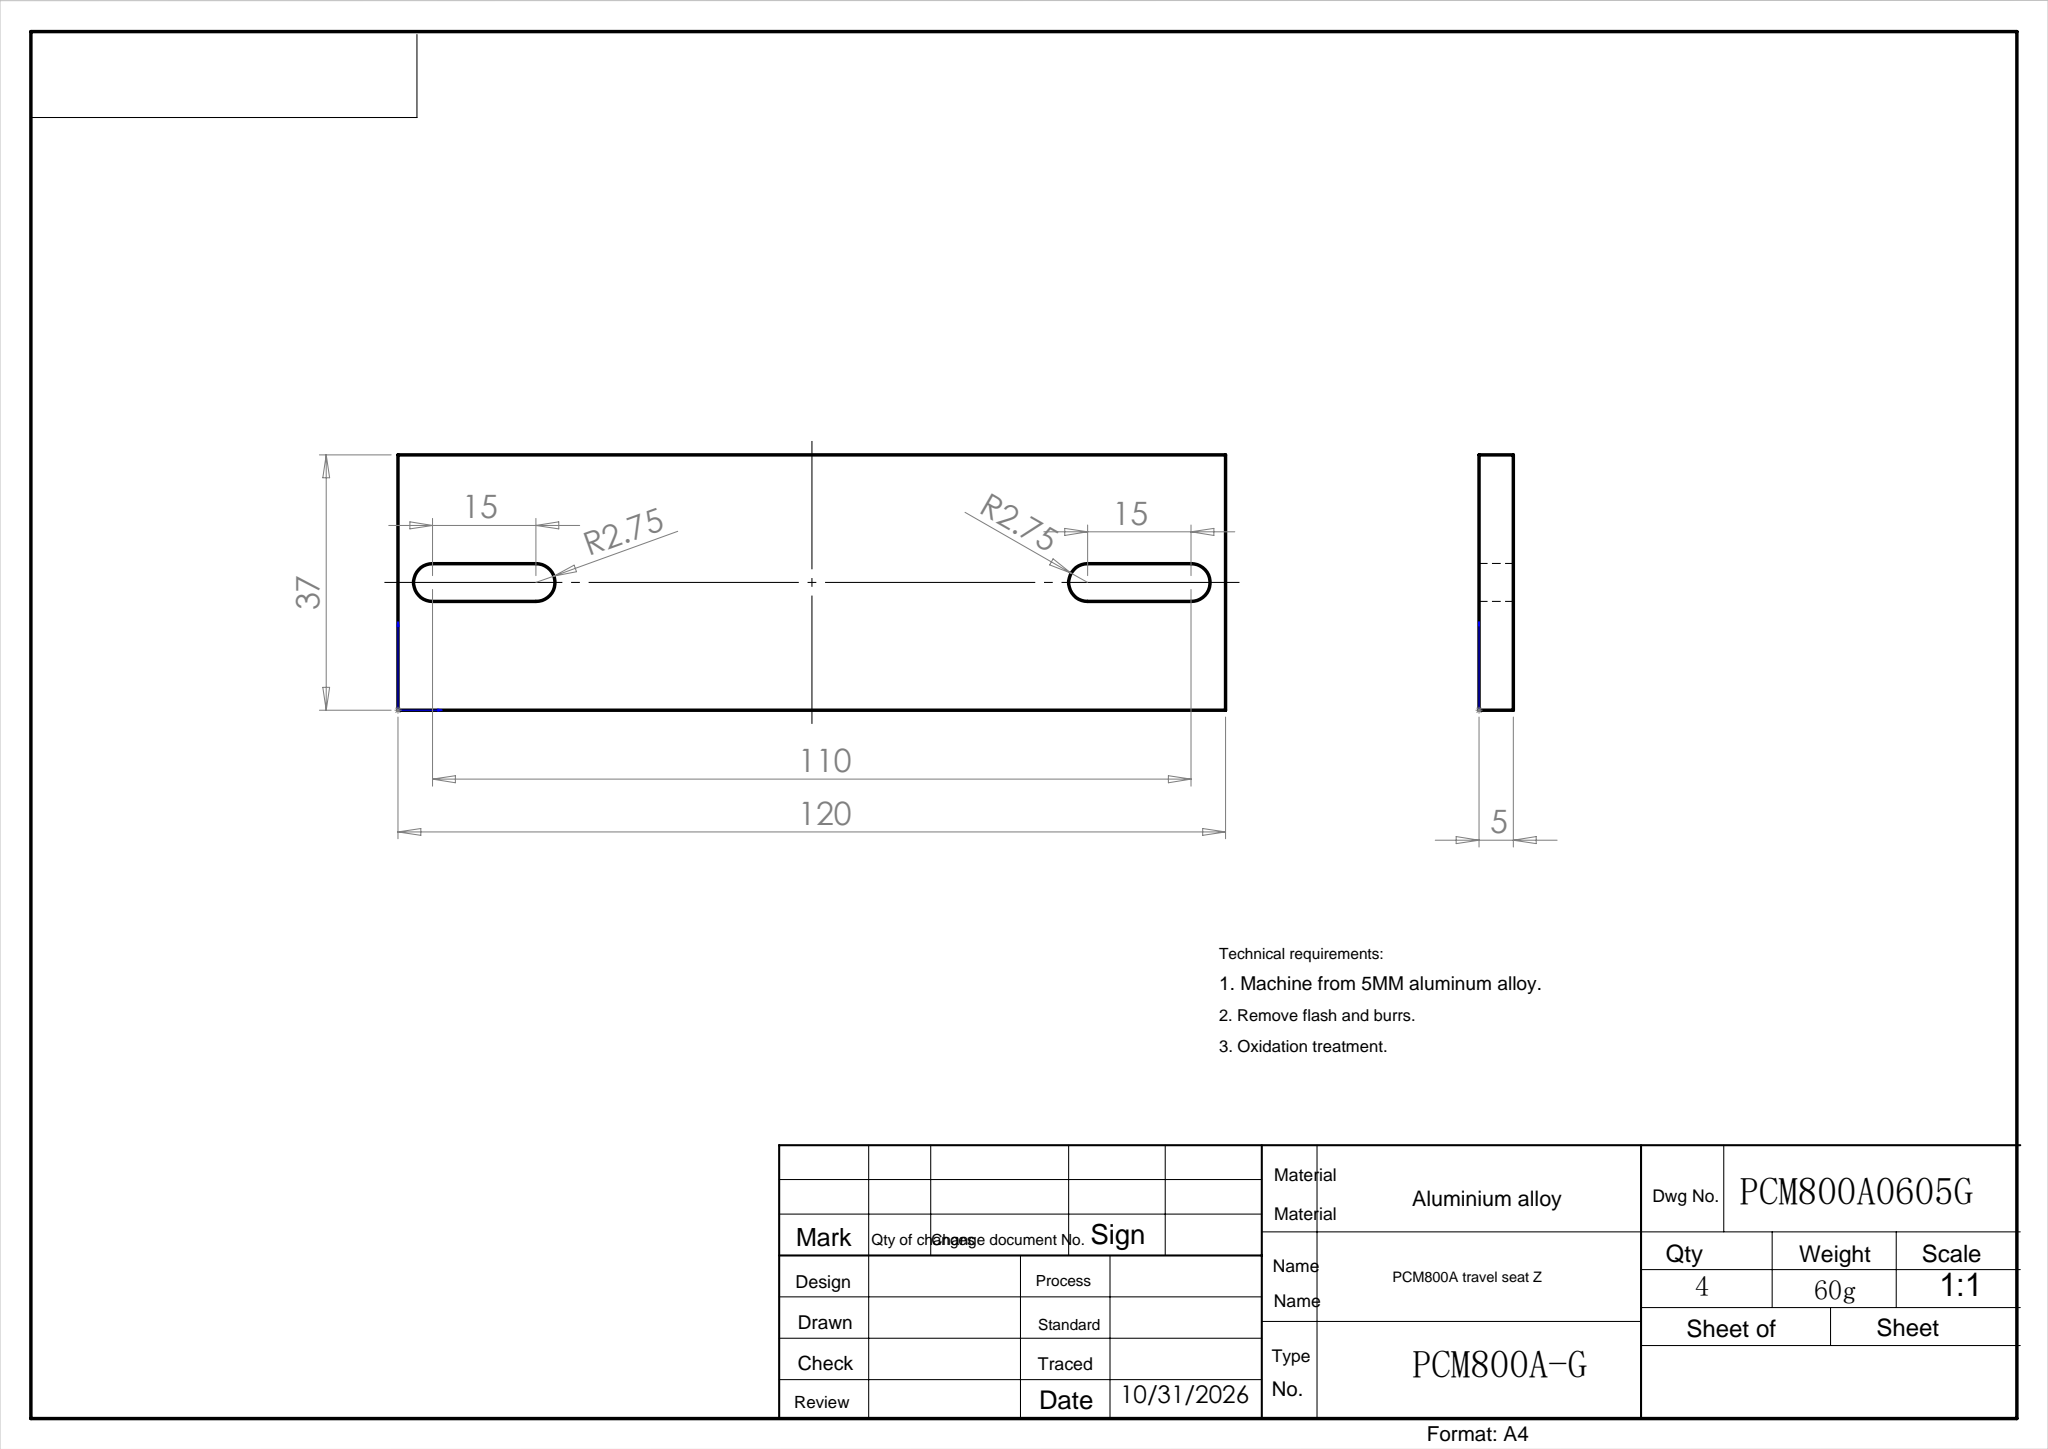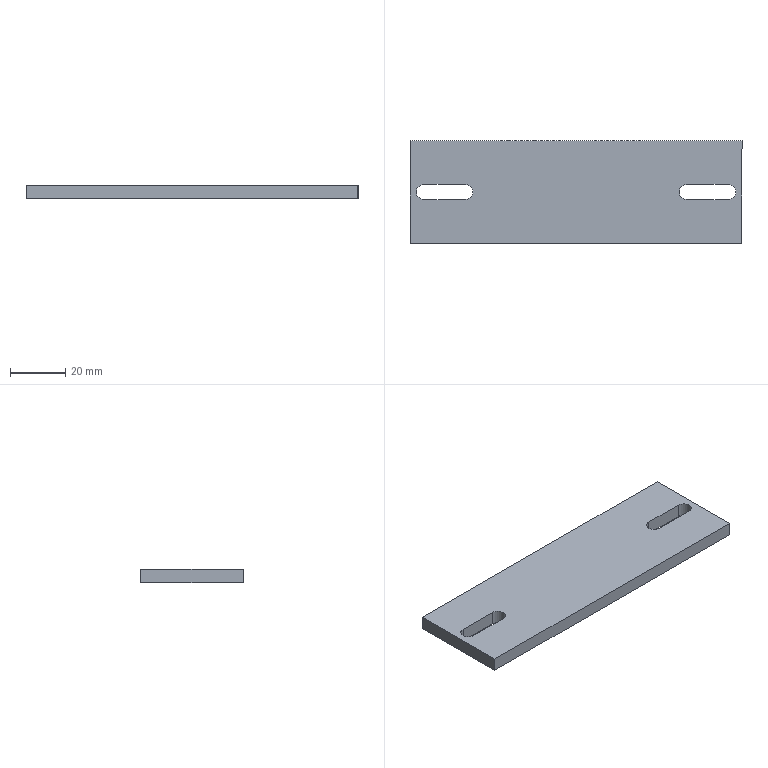Part | SolidWorks | features Extrusion 1 | 1 solid | 16 faces | box 120 x 37 x 5 mm | volume 21137 mm3 | plane 10 | cylinder 6 | commonest cylinder face diameters 5.5 x6
STEP:
#1=CARTESIAN_POINT('',(5.,21.25,5.));
#2=VERTEX_POINT('',#1);
#3=CARTESIAN_POINT('',(2.25,18.5,5.));
#4=VERTEX_POINT('',#3);
#5=CARTESIAN_POINT('',(5.,18.5,5.));
#6=DIRECTION('',(0.,0.,1.));
#7=DIRECTION('',(1.,0.,0.));
#8=AXIS2_PLACEMENT_3D('',#5,#6,#7);
#9=CIRCLE('',#8,2.75);
#10=EDGE_CURVE('',#2,#4,#9,.T.);
#11=ORIENTED_EDGE('',*,*,#10,.T.);
#12=CARTESIAN_POINT('',(2.25,18.5,0.));
#13=VERTEX_POINT('',#12);
#14=CARTESIAN_POINT('',(2.25,18.5,5.));
#15=DIRECTION('',(0.,0.,-1.));
#16=VECTOR('',#15,1000.);
#17=LINE('',#14,#16);
#18=EDGE_CURVE('',#4,#13,#17,.T.);
#19=ORIENTED_EDGE('',*,*,#18,.T.);
#20=CARTESIAN_POINT('',(5.,21.25,0.));
#21=VERTEX_POINT('',#20);
#22=CARTESIAN_POINT('',(5.,18.5,0.));
#23=DIRECTION('',(0.,0.,1.));
#24=DIRECTION('',(1.,0.,0.));
#25=AXIS2_PLACEMENT_3D('',#22,#23,#24);
#26=CIRCLE('',#25,2.75);
#27=EDGE_CURVE('',#21,#13,#26,.T.);
#28=ORIENTED_EDGE('',*,*,#27,.F.);
#29=CARTESIAN_POINT('',(5.,21.25,5.));
#30=DIRECTION('',(0.,0.,-1.));
#31=VECTOR('',#30,1000.);
#32=LINE('',#29,#31);
#33=EDGE_CURVE('',#2,#21,#32,.T.);
#34=ORIENTED_EDGE('',*,*,#33,.F.);
#35=EDGE_LOOP('',(#11,#19,#28,#34));
#36=FACE_OUTER_BOUND('',#35,.T.);
#37=CARTESIAN_POINT('',(5.,18.5,5.));
#38=DIRECTION('',(0.,0.,-1.));
#39=DIRECTION('',(-1.,0.,0.));
#40=AXIS2_PLACEMENT_3D('',#37,#38,#39);
#41=CYLINDRICAL_SURFACE('',#40,2.75);
#42=ADVANCED_FACE('',(#36),#41,.F.);
#43=CARTESIAN_POINT('',(100.,21.25,5.));
#44=VERTEX_POINT('',#43);
#45=CARTESIAN_POINT('',(97.25,18.5,5.));
#46=VERTEX_POINT('',#45);
#47=CARTESIAN_POINT('',(100.,18.5,5.));
#48=DIRECTION('',(0.,0.,1.));
#49=DIRECTION('',(-1.,0.,0.));
#50=AXIS2_PLACEMENT_3D('',#47,#48,#49);
#51=CIRCLE('',#50,2.75);
#52=EDGE_CURVE('',#44,#46,#51,.T.);
#53=ORIENTED_EDGE('',*,*,#52,.T.);
#54=CARTESIAN_POINT('',(97.25,18.5,0.));
#55=VERTEX_POINT('',#54);
#56=CARTESIAN_POINT('',(97.25,18.5,5.));
#57=DIRECTION('',(0.,0.,-1.));
#58=VECTOR('',#57,1000.);
#59=LINE('',#56,#58);
#60=EDGE_CURVE('',#46,#55,#59,.T.);
#61=ORIENTED_EDGE('',*,*,#60,.T.);
#62=CARTESIAN_POINT('',(100.,21.25,0.));
#63=VERTEX_POINT('',#62);
#64=CARTESIAN_POINT('',(100.,18.5,0.));
#65=DIRECTION('',(0.,0.,1.));
#66=DIRECTION('',(-1.,0.,0.));
#67=AXIS2_PLACEMENT_3D('',#64,#65,#66);
#68=CIRCLE('',#67,2.75);
#69=EDGE_CURVE('',#63,#55,#68,.T.);
#70=ORIENTED_EDGE('',*,*,#69,.F.);
#71=CARTESIAN_POINT('',(100.,21.25,5.));
#72=DIRECTION('',(0.,0.,-1.));
#73=VECTOR('',#72,1000.);
#74=LINE('',#71,#73);
#75=EDGE_CURVE('',#44,#63,#74,.T.);
#76=ORIENTED_EDGE('',*,*,#75,.F.);
#77=EDGE_LOOP('',(#53,#61,#70,#76));
#78=FACE_OUTER_BOUND('',#77,.T.);
#79=CARTESIAN_POINT('',(100.,18.5,5.));
#80=DIRECTION('',(0.,0.,-1.));
#81=DIRECTION('',(-1.,0.,0.));
#82=AXIS2_PLACEMENT_3D('',#79,#80,#81);
#83=CYLINDRICAL_SURFACE('',#82,2.75);
#84=ADVANCED_FACE('',(#78),#83,.F.);
#85=ORIENTED_EDGE('',*,*,#52,.F.);
#86=CARTESIAN_POINT('',(115.,21.25,5.));
#87=VERTEX_POINT('',#86);
#88=CARTESIAN_POINT('',(115.,21.25,5.));
#89=DIRECTION('',(-1.,0.,0.));
#90=VECTOR('',#89,1000.);
#91=LINE('',#88,#90);
#92=EDGE_CURVE('',#87,#44,#91,.T.);
#93=ORIENTED_EDGE('',*,*,#92,.F.);
#94=CARTESIAN_POINT('',(115.,15.75,5.));
#95=VERTEX_POINT('',#94);
#96=CARTESIAN_POINT('',(115.,18.5,5.));
#97=DIRECTION('',(0.,0.,1.));
#98=DIRECTION('',(-1.,0.,0.));
#99=AXIS2_PLACEMENT_3D('',#96,#97,#98);
#100=CIRCLE('',#99,2.75);
#101=EDGE_CURVE('',#95,#87,#100,.T.);
#102=ORIENTED_EDGE('',*,*,#101,.F.);
#103=CARTESIAN_POINT('',(100.,15.75,5.));
#104=VERTEX_POINT('',#103);
#105=CARTESIAN_POINT('',(115.,15.75,5.));
#106=DIRECTION('',(1.,0.,0.));
#107=VECTOR('',#106,1000.);
#108=LINE('',#105,#107);
#109=EDGE_CURVE('',#104,#95,#108,.T.);
#110=ORIENTED_EDGE('',*,*,#109,.F.);
#111=CARTESIAN_POINT('',(100.,18.5,5.));
#112=DIRECTION('',(0.,0.,1.));
#113=DIRECTION('',(-1.,0.,0.));
#114=AXIS2_PLACEMENT_3D('',#111,#112,#113);
#115=CIRCLE('',#114,2.75);
#116=EDGE_CURVE('',#46,#104,#115,.T.);
#117=ORIENTED_EDGE('',*,*,#116,.F.);
#118=EDGE_LOOP('',(#85,#93,#102,#110,#117));
#119=FACE_BOUND('',#118,.T.);
#120=CARTESIAN_POINT('',(0.,37.,5.));
#121=VERTEX_POINT('',#120);
#122=CARTESIAN_POINT('',(0.,0.,5.));
#123=VERTEX_POINT('',#122);
#124=CARTESIAN_POINT('',(0.,0.,5.));
#125=DIRECTION('',(0.,-1.,0.));
#126=VECTOR('',#125,1000.);
#127=LINE('',#124,#126);
#128=EDGE_CURVE('',#121,#123,#127,.T.);
#129=ORIENTED_EDGE('',*,*,#128,.T.);
#130=CARTESIAN_POINT('',(120.,0.,5.));
#131=VERTEX_POINT('',#130);
#132=CARTESIAN_POINT('',(0.,0.,5.));
#133=DIRECTION('',(1.,0.,0.));
#134=VECTOR('',#133,1000.);
#135=LINE('',#132,#134);
#136=EDGE_CURVE('',#123,#131,#135,.T.);
#137=ORIENTED_EDGE('',*,*,#136,.T.);
#138=CARTESIAN_POINT('',(120.,37.,5.));
#139=VERTEX_POINT('',#138);
#140=CARTESIAN_POINT('',(120.,0.,5.));
#141=DIRECTION('',(0.,1.,0.));
#142=VECTOR('',#141,1000.);
#143=LINE('',#140,#142);
#144=EDGE_CURVE('',#131,#139,#143,.T.);
#145=ORIENTED_EDGE('',*,*,#144,.T.);
#146=CARTESIAN_POINT('',(0.,37.,5.));
#147=DIRECTION('',(-1.,0.,0.));
#148=VECTOR('',#147,1000.);
#149=LINE('',#146,#148);
#150=EDGE_CURVE('',#139,#121,#149,.T.);
#151=ORIENTED_EDGE('',*,*,#150,.T.);
#152=EDGE_LOOP('',(#129,#137,#145,#151));
#153=FACE_OUTER_BOUND('',#152,.T.);
#154=ORIENTED_EDGE('',*,*,#10,.F.);
#155=CARTESIAN_POINT('',(20.,21.25,5.));
#156=VERTEX_POINT('',#155);
#157=CARTESIAN_POINT('',(5.,21.25,5.));
#158=DIRECTION('',(-1.,0.,0.));
#159=VECTOR('',#158,1000.);
#160=LINE('',#157,#159);
#161=EDGE_CURVE('',#156,#2,#160,.T.);
#162=ORIENTED_EDGE('',*,*,#161,.F.);
#163=CARTESIAN_POINT('',(20.,15.75,5.));
#164=VERTEX_POINT('',#163);
#165=CARTESIAN_POINT('',(20.,18.5,5.));
#166=DIRECTION('',(0.,0.,1.));
#167=DIRECTION('',(1.,0.,0.));
#168=AXIS2_PLACEMENT_3D('',#165,#166,#167);
#169=CIRCLE('',#168,2.75);
#170=EDGE_CURVE('',#164,#156,#169,.T.);
#171=ORIENTED_EDGE('',*,*,#170,.F.);
#172=CARTESIAN_POINT('',(5.,15.75,5.));
#173=VERTEX_POINT('',#172);
#174=CARTESIAN_POINT('',(5.,15.75,5.));
#175=DIRECTION('',(1.,0.,0.));
#176=VECTOR('',#175,1000.);
#177=LINE('',#174,#176);
#178=EDGE_CURVE('',#173,#164,#177,.T.);
#179=ORIENTED_EDGE('',*,*,#178,.F.);
#180=CARTESIAN_POINT('',(5.,18.5,5.));
#181=DIRECTION('',(0.,0.,1.));
#182=DIRECTION('',(1.,0.,0.));
#183=AXIS2_PLACEMENT_3D('',#180,#181,#182);
#184=CIRCLE('',#183,2.75);
#185=EDGE_CURVE('',#4,#173,#184,.T.);
#186=ORIENTED_EDGE('',*,*,#185,.F.);
#187=EDGE_LOOP('',(#154,#162,#171,#179,#186));
#188=FACE_BOUND('',#187,.T.);
#189=CARTESIAN_POINT('',(0.,37.,5.));
#190=DIRECTION('',(0.,0.,-1.));
#191=DIRECTION('',(-1.,0.,0.));
#192=AXIS2_PLACEMENT_3D('',#189,#190,#191);
#193=PLANE('',#192);
#194=ADVANCED_FACE('',(#119,#153,#188),#193,.F.);
#195=CARTESIAN_POINT('',(115.,21.25,0.));
#196=VERTEX_POINT('',#195);
#197=CARTESIAN_POINT('',(115.,21.25,0.));
#198=DIRECTION('',(-1.,0.,0.));
#199=VECTOR('',#198,1000.);
#200=LINE('',#197,#199);
#201=EDGE_CURVE('',#196,#63,#200,.T.);
#202=ORIENTED_EDGE('',*,*,#201,.T.);
#203=ORIENTED_EDGE('',*,*,#69,.T.);
#204=CARTESIAN_POINT('',(100.,15.75,0.));
#205=VERTEX_POINT('',#204);
#206=CARTESIAN_POINT('',(100.,18.5,0.));
#207=DIRECTION('',(0.,0.,1.));
#208=DIRECTION('',(-1.,0.,0.));
#209=AXIS2_PLACEMENT_3D('',#206,#207,#208);
#210=CIRCLE('',#209,2.75);
#211=EDGE_CURVE('',#55,#205,#210,.T.);
#212=ORIENTED_EDGE('',*,*,#211,.T.);
#213=CARTESIAN_POINT('',(115.,15.75,0.));
#214=VERTEX_POINT('',#213);
#215=CARTESIAN_POINT('',(115.,15.75,0.));
#216=DIRECTION('',(1.,0.,0.));
#217=VECTOR('',#216,1000.);
#218=LINE('',#215,#217);
#219=EDGE_CURVE('',#205,#214,#218,.T.);
#220=ORIENTED_EDGE('',*,*,#219,.T.);
#221=CARTESIAN_POINT('',(115.,18.5,0.));
#222=DIRECTION('',(0.,0.,1.));
#223=DIRECTION('',(-1.,0.,0.));
#224=AXIS2_PLACEMENT_3D('',#221,#222,#223);
#225=CIRCLE('',#224,2.75);
#226=EDGE_CURVE('',#214,#196,#225,.T.);
#227=ORIENTED_EDGE('',*,*,#226,.T.);
#228=EDGE_LOOP('',(#202,#203,#212,#220,#227));
#229=FACE_BOUND('',#228,.T.);
#230=CARTESIAN_POINT('',(0.,37.,0.));
#231=VERTEX_POINT('',#230);
#232=CARTESIAN_POINT('',(0.,0.,0.));
#233=VERTEX_POINT('',#232);
#234=CARTESIAN_POINT('',(0.,0.,0.));
#235=DIRECTION('',(0.,-1.,0.));
#236=VECTOR('',#235,1000.);
#237=LINE('',#234,#236);
#238=EDGE_CURVE('',#231,#233,#237,.T.);
#239=ORIENTED_EDGE('',*,*,#238,.F.);
#240=CARTESIAN_POINT('',(120.,37.,0.));
#241=VERTEX_POINT('',#240);
#242=CARTESIAN_POINT('',(0.,37.,0.));
#243=DIRECTION('',(-1.,0.,0.));
#244=VECTOR('',#243,1000.);
#245=LINE('',#242,#244);
#246=EDGE_CURVE('',#241,#231,#245,.T.);
#247=ORIENTED_EDGE('',*,*,#246,.F.);
#248=CARTESIAN_POINT('',(120.,0.,0.));
#249=VERTEX_POINT('',#248);
#250=CARTESIAN_POINT('',(120.,0.,0.));
#251=DIRECTION('',(0.,1.,0.));
#252=VECTOR('',#251,1000.);
#253=LINE('',#250,#252);
#254=EDGE_CURVE('',#249,#241,#253,.T.);
#255=ORIENTED_EDGE('',*,*,#254,.F.);
#256=CARTESIAN_POINT('',(0.,0.,0.));
#257=DIRECTION('',(1.,0.,0.));
#258=VECTOR('',#257,1000.);
#259=LINE('',#256,#258);
#260=EDGE_CURVE('',#233,#249,#259,.T.);
#261=ORIENTED_EDGE('',*,*,#260,.F.);
#262=EDGE_LOOP('',(#239,#247,#255,#261));
#263=FACE_OUTER_BOUND('',#262,.T.);
#264=CARTESIAN_POINT('',(20.,21.25,0.));
#265=VERTEX_POINT('',#264);
#266=CARTESIAN_POINT('',(5.,21.25,0.));
#267=DIRECTION('',(-1.,0.,0.));
#268=VECTOR('',#267,1000.);
#269=LINE('',#266,#268);
#270=EDGE_CURVE('',#265,#21,#269,.T.);
#271=ORIENTED_EDGE('',*,*,#270,.T.);
#272=ORIENTED_EDGE('',*,*,#27,.T.);
#273=CARTESIAN_POINT('',(5.,15.75,0.));
#274=VERTEX_POINT('',#273);
#275=CARTESIAN_POINT('',(5.,18.5,0.));
#276=DIRECTION('',(0.,0.,1.));
#277=DIRECTION('',(1.,0.,0.));
#278=AXIS2_PLACEMENT_3D('',#275,#276,#277);
#279=CIRCLE('',#278,2.75);
#280=EDGE_CURVE('',#13,#274,#279,.T.);
#281=ORIENTED_EDGE('',*,*,#280,.T.);
#282=CARTESIAN_POINT('',(20.,15.75,0.));
#283=VERTEX_POINT('',#282);
#284=CARTESIAN_POINT('',(5.,15.75,0.));
#285=DIRECTION('',(1.,0.,0.));
#286=VECTOR('',#285,1000.);
#287=LINE('',#284,#286);
#288=EDGE_CURVE('',#274,#283,#287,.T.);
#289=ORIENTED_EDGE('',*,*,#288,.T.);
#290=CARTESIAN_POINT('',(20.,18.5,0.));
#291=DIRECTION('',(0.,0.,1.));
#292=DIRECTION('',(1.,0.,0.));
#293=AXIS2_PLACEMENT_3D('',#290,#291,#292);
#294=CIRCLE('',#293,2.75);
#295=EDGE_CURVE('',#283,#265,#294,.T.);
#296=ORIENTED_EDGE('',*,*,#295,.T.);
#297=EDGE_LOOP('',(#271,#272,#281,#289,#296));
#298=FACE_BOUND('',#297,.T.);
#299=CARTESIAN_POINT('',(0.,37.,0.));
#300=DIRECTION('',(0.,0.,-1.));
#301=DIRECTION('',(-1.,0.,0.));
#302=AXIS2_PLACEMENT_3D('',#299,#300,#301);
#303=PLANE('',#302);
#304=ADVANCED_FACE('',(#229,#263,#298),#303,.T.);
#305=ORIENTED_EDGE('',*,*,#238,.T.);
#306=CARTESIAN_POINT('',(0.,0.,5.));
#307=DIRECTION('',(0.,0.,-1.));
#308=VECTOR('',#307,1000.);
#309=LINE('',#306,#308);
#310=EDGE_CURVE('',#123,#233,#309,.T.);
#311=ORIENTED_EDGE('',*,*,#310,.F.);
#312=ORIENTED_EDGE('',*,*,#128,.F.);
#313=CARTESIAN_POINT('',(0.,37.,5.));
#314=DIRECTION('',(0.,0.,-1.));
#315=VECTOR('',#314,1000.);
#316=LINE('',#313,#315);
#317=EDGE_CURVE('',#121,#231,#316,.T.);
#318=ORIENTED_EDGE('',*,*,#317,.T.);
#319=EDGE_LOOP('',(#305,#311,#312,#318));
#320=FACE_OUTER_BOUND('',#319,.T.);
#321=CARTESIAN_POINT('',(0.,0.,5.));
#322=DIRECTION('',(1.,0.,0.));
#323=DIRECTION('',(0.,0.,-1.));
#324=AXIS2_PLACEMENT_3D('',#321,#322,#323);
#325=PLANE('',#324);
#326=ADVANCED_FACE('',(#320),#325,.F.);
#327=ORIENTED_EDGE('',*,*,#260,.T.);
#328=CARTESIAN_POINT('',(120.,0.,5.));
#329=DIRECTION('',(0.,0.,-1.));
#330=VECTOR('',#329,1000.);
#331=LINE('',#328,#330);
#332=EDGE_CURVE('',#131,#249,#331,.T.);
#333=ORIENTED_EDGE('',*,*,#332,.F.);
#334=ORIENTED_EDGE('',*,*,#136,.F.);
#335=ORIENTED_EDGE('',*,*,#310,.T.);
#336=EDGE_LOOP('',(#327,#333,#334,#335));
#337=FACE_OUTER_BOUND('',#336,.T.);
#338=CARTESIAN_POINT('',(0.,0.,5.));
#339=DIRECTION('',(0.,1.,0.));
#340=DIRECTION('',(0.,0.,1.));
#341=AXIS2_PLACEMENT_3D('',#338,#339,#340);
#342=PLANE('',#341);
#343=ADVANCED_FACE('',(#337),#342,.F.);
#344=ORIENTED_EDGE('',*,*,#254,.T.);
#345=CARTESIAN_POINT('',(120.,37.,5.));
#346=DIRECTION('',(0.,0.,-1.));
#347=VECTOR('',#346,1000.);
#348=LINE('',#345,#347);
#349=EDGE_CURVE('',#139,#241,#348,.T.);
#350=ORIENTED_EDGE('',*,*,#349,.F.);
#351=ORIENTED_EDGE('',*,*,#144,.F.);
#352=ORIENTED_EDGE('',*,*,#332,.T.);
#353=EDGE_LOOP('',(#344,#350,#351,#352));
#354=FACE_OUTER_BOUND('',#353,.T.);
#355=CARTESIAN_POINT('',(120.,0.,5.));
#356=DIRECTION('',(-1.,0.,0.));
#357=DIRECTION('',(0.,-1.,0.));
#358=AXIS2_PLACEMENT_3D('',#355,#356,#357);
#359=PLANE('',#358);
#360=ADVANCED_FACE('',(#354),#359,.F.);
#361=ORIENTED_EDGE('',*,*,#246,.T.);
#362=ORIENTED_EDGE('',*,*,#317,.F.);
#363=ORIENTED_EDGE('',*,*,#150,.F.);
#364=ORIENTED_EDGE('',*,*,#349,.T.);
#365=EDGE_LOOP('',(#361,#362,#363,#364));
#366=FACE_OUTER_BOUND('',#365,.T.);
#367=CARTESIAN_POINT('',(0.,37.,5.));
#368=DIRECTION('',(0.,-1.,0.));
#369=DIRECTION('',(0.,0.,-1.));
#370=AXIS2_PLACEMENT_3D('',#367,#368,#369);
#371=PLANE('',#370);
#372=ADVANCED_FACE('',(#366),#371,.F.);
#373=ORIENTED_EDGE('',*,*,#60,.F.);
#374=ORIENTED_EDGE('',*,*,#116,.T.);
#375=CARTESIAN_POINT('',(100.,15.75,5.));
#376=DIRECTION('',(0.,0.,-1.));
#377=VECTOR('',#376,1000.);
#378=LINE('',#375,#377);
#379=EDGE_CURVE('',#104,#205,#378,.T.);
#380=ORIENTED_EDGE('',*,*,#379,.T.);
#381=ORIENTED_EDGE('',*,*,#211,.F.);
#382=EDGE_LOOP('',(#373,#374,#380,#381));
#383=FACE_OUTER_BOUND('',#382,.T.);
#384=CARTESIAN_POINT('',(100.,18.5,5.));
#385=DIRECTION('',(0.,0.,-1.));
#386=DIRECTION('',(-1.,0.,0.));
#387=AXIS2_PLACEMENT_3D('',#384,#385,#386);
#388=CYLINDRICAL_SURFACE('',#387,2.75);
#389=ADVANCED_FACE('',(#383),#388,.F.);
#390=ORIENTED_EDGE('',*,*,#219,.F.);
#391=ORIENTED_EDGE('',*,*,#379,.F.);
#392=ORIENTED_EDGE('',*,*,#109,.T.);
#393=CARTESIAN_POINT('',(115.,15.75,5.));
#394=DIRECTION('',(0.,0.,-1.));
#395=VECTOR('',#394,1000.);
#396=LINE('',#393,#395);
#397=EDGE_CURVE('',#95,#214,#396,.T.);
#398=ORIENTED_EDGE('',*,*,#397,.T.);
#399=EDGE_LOOP('',(#390,#391,#392,#398));
#400=FACE_OUTER_BOUND('',#399,.T.);
#401=CARTESIAN_POINT('',(115.,15.75,5.));
#402=DIRECTION('',(0.,1.,0.));
#403=DIRECTION('',(0.,0.,1.));
#404=AXIS2_PLACEMENT_3D('',#401,#402,#403);
#405=PLANE('',#404);
#406=ADVANCED_FACE('',(#400),#405,.T.);
#407=ORIENTED_EDGE('',*,*,#226,.F.);
#408=ORIENTED_EDGE('',*,*,#397,.F.);
#409=ORIENTED_EDGE('',*,*,#101,.T.);
#410=CARTESIAN_POINT('',(115.,21.25,5.));
#411=DIRECTION('',(0.,0.,-1.));
#412=VECTOR('',#411,1000.);
#413=LINE('',#410,#412);
#414=EDGE_CURVE('',#87,#196,#413,.T.);
#415=ORIENTED_EDGE('',*,*,#414,.T.);
#416=EDGE_LOOP('',(#407,#408,#409,#415));
#417=FACE_OUTER_BOUND('',#416,.T.);
#418=CARTESIAN_POINT('',(115.,18.5,5.));
#419=DIRECTION('',(0.,0.,-1.));
#420=DIRECTION('',(-1.,0.,0.));
#421=AXIS2_PLACEMENT_3D('',#418,#419,#420);
#422=CYLINDRICAL_SURFACE('',#421,2.75);
#423=ADVANCED_FACE('',(#417),#422,.F.);
#424=ORIENTED_EDGE('',*,*,#201,.F.);
#425=ORIENTED_EDGE('',*,*,#414,.F.);
#426=ORIENTED_EDGE('',*,*,#92,.T.);
#427=ORIENTED_EDGE('',*,*,#75,.T.);
#428=EDGE_LOOP('',(#424,#425,#426,#427));
#429=FACE_OUTER_BOUND('',#428,.T.);
#430=CARTESIAN_POINT('',(115.,21.25,5.));
#431=DIRECTION('',(0.,-1.,0.));
#432=DIRECTION('',(0.,0.,-1.));
#433=AXIS2_PLACEMENT_3D('',#430,#431,#432);
#434=PLANE('',#433);
#435=ADVANCED_FACE('',(#429),#434,.T.);
#436=ORIENTED_EDGE('',*,*,#18,.F.);
#437=ORIENTED_EDGE('',*,*,#185,.T.);
#438=CARTESIAN_POINT('',(5.,15.75,5.));
#439=DIRECTION('',(0.,0.,-1.));
#440=VECTOR('',#439,1000.);
#441=LINE('',#438,#440);
#442=EDGE_CURVE('',#173,#274,#441,.T.);
#443=ORIENTED_EDGE('',*,*,#442,.T.);
#444=ORIENTED_EDGE('',*,*,#280,.F.);
#445=EDGE_LOOP('',(#436,#437,#443,#444));
#446=FACE_OUTER_BOUND('',#445,.T.);
#447=CARTESIAN_POINT('',(5.,18.5,5.));
#448=DIRECTION('',(0.,0.,-1.));
#449=DIRECTION('',(-1.,0.,0.));
#450=AXIS2_PLACEMENT_3D('',#447,#448,#449);
#451=CYLINDRICAL_SURFACE('',#450,2.75);
#452=ADVANCED_FACE('',(#446),#451,.F.);
#453=ORIENTED_EDGE('',*,*,#288,.F.);
#454=ORIENTED_EDGE('',*,*,#442,.F.);
#455=ORIENTED_EDGE('',*,*,#178,.T.);
#456=CARTESIAN_POINT('',(20.,15.75,5.));
#457=DIRECTION('',(0.,0.,-1.));
#458=VECTOR('',#457,1000.);
#459=LINE('',#456,#458);
#460=EDGE_CURVE('',#164,#283,#459,.T.);
#461=ORIENTED_EDGE('',*,*,#460,.T.);
#462=EDGE_LOOP('',(#453,#454,#455,#461));
#463=FACE_OUTER_BOUND('',#462,.T.);
#464=CARTESIAN_POINT('',(5.,15.75,5.));
#465=DIRECTION('',(0.,1.,0.));
#466=DIRECTION('',(0.,0.,1.));
#467=AXIS2_PLACEMENT_3D('',#464,#465,#466);
#468=PLANE('',#467);
#469=ADVANCED_FACE('',(#463),#468,.T.);
#470=ORIENTED_EDGE('',*,*,#295,.F.);
#471=ORIENTED_EDGE('',*,*,#460,.F.);
#472=ORIENTED_EDGE('',*,*,#170,.T.);
#473=CARTESIAN_POINT('',(20.,21.25,5.));
#474=DIRECTION('',(0.,0.,-1.));
#475=VECTOR('',#474,1000.);
#476=LINE('',#473,#475);
#477=EDGE_CURVE('',#156,#265,#476,.T.);
#478=ORIENTED_EDGE('',*,*,#477,.T.);
#479=EDGE_LOOP('',(#470,#471,#472,#478));
#480=FACE_OUTER_BOUND('',#479,.T.);
#481=CARTESIAN_POINT('',(20.,18.5,5.));
#482=DIRECTION('',(0.,0.,-1.));
#483=DIRECTION('',(-1.,0.,0.));
#484=AXIS2_PLACEMENT_3D('',#481,#482,#483);
#485=CYLINDRICAL_SURFACE('',#484,2.75);
#486=ADVANCED_FACE('',(#480),#485,.F.);
#487=ORIENTED_EDGE('',*,*,#270,.F.);
#488=ORIENTED_EDGE('',*,*,#477,.F.);
#489=ORIENTED_EDGE('',*,*,#161,.T.);
#490=ORIENTED_EDGE('',*,*,#33,.T.);
#491=EDGE_LOOP('',(#487,#488,#489,#490));
#492=FACE_OUTER_BOUND('',#491,.T.);
#493=CARTESIAN_POINT('',(5.,21.25,5.));
#494=DIRECTION('',(0.,-1.,0.));
#495=DIRECTION('',(0.,0.,-1.));
#496=AXIS2_PLACEMENT_3D('',#493,#494,#495);
#497=PLANE('',#496);
#498=ADVANCED_FACE('',(#492),#497,.T.);
#499=CLOSED_SHELL('',(#42,#84,#194,#304,#326,#343,#360,#372,#389,#406,#423,#435,#452,#469,#486,#498));
#500=MANIFOLD_SOLID_BREP('',#499);
#501=CARTESIAN_POINT('',(0.,0.,0.));
#502=DIRECTION('',(0.,0.,1.));
#503=DIRECTION('',(1.,0.,0.));
#504=AXIS2_PLACEMENT_3D('',#501,#502,#503);
#505=(LENGTH_UNIT()NAMED_UNIT(*)SI_UNIT(.MILLI.,.METRE.));
#506=UNCERTAINTY_MEASURE_WITH_UNIT(LENGTH_MEASURE(0.00001),#505,'','');
#507=(NAMED_UNIT(*)PLANE_ANGLE_UNIT()SI_UNIT($,.RADIAN.));
#508=(NAMED_UNIT(*)SI_UNIT($,.STERADIAN.)SOLID_ANGLE_UNIT());
#509=(GEOMETRIC_REPRESENTATION_CONTEXT(3)GLOBAL_UNCERTAINTY_ASSIGNED_CONTEXT((#506))GLOBAL_UNIT_ASSIGNED_CONTEXT((#505,#507,#508))REPRESENTATION_CONTEXT('',''));
#510=ADVANCED_BREP_SHAPE_REPRESENTATION('',(#500,#504),#509);